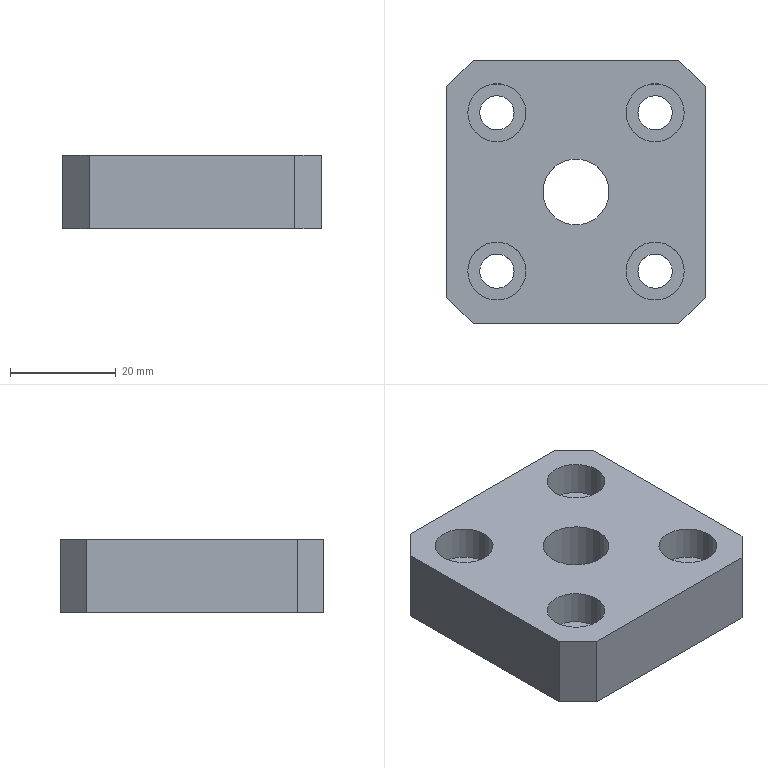Part | STEP file | BU-A01-2 | 1 solid | 32 faces | box 49 x 50 x 14 mm | volume 28416 mm3 | cylinder 18 | plane 14 | commonest cylinder face diameters 6.5 x8 11 x8 12.5 x2